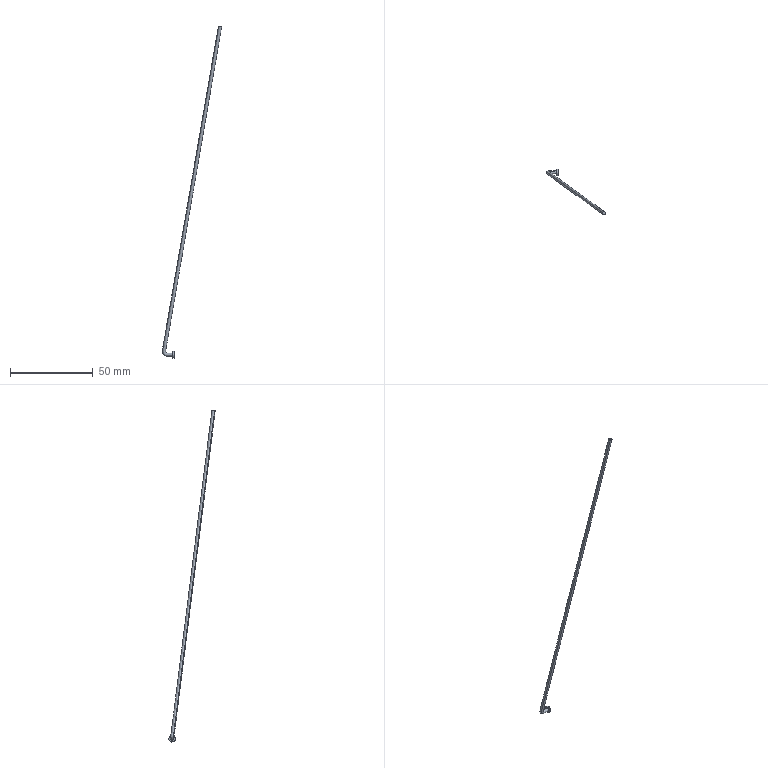Part | STEP file | BREP_61 | 1 solid | 7 faces | box 35.925 x 28.108 x 200.702 mm | volume 653.861 mm3 | plane 3 | spline 2 | cylinder 2 | commonest cylinder face diameters 4 x2
STEP:
#1=CARTESIAN_POINT('',(0.,0.,0.));
#2=DIRECTION('',(0.,0.,1.));
#3=DIRECTION('',(1.,0.,0.));
#4=AXIS2_PLACEMENT_3D('',#1,#2,#3);
#5=CARTESIAN_POINT('',(-13.811,0.6169,212.934));
#6=VERTEX_POINT('',#5);
#7=CARTESIAN_POINT('',(-43.38,25.615,15.366));
#8=VERTEX_POINT('',#7);
#9=CARTESIAN_POINT('',(-13.811,0.6169,212.934));
#10=CARTESIAN_POINT('',(-14.915,1.425,206.549));
#11=CARTESIAN_POINT('',(-17.123,3.041,193.777));
#12=CARTESIAN_POINT('',(-20.435,5.465,174.62));
#13=CARTESIAN_POINT('',(-23.747,7.889,155.462));
#14=CARTESIAN_POINT('',(-27.059,10.313,136.305));
#15=CARTESIAN_POINT('',(-30.371,12.737,117.147));
#16=CARTESIAN_POINT('',(-34.787,15.969,91.603));
#17=CARTESIAN_POINT('',(-38.375,18.594,70.85));
#18=CARTESIAN_POINT('',(-41.135,20.614,54.885));
#19=CARTESIAN_POINT('',(-41.963,21.22,50.096));
#20=CARTESIAN_POINT('',(-42.791,21.826,45.306));
#21=CARTESIAN_POINT('',(-43.619,22.432,40.517));
#22=CARTESIAN_POINT('',(-44.447,23.038,35.728));
#23=CARTESIAN_POINT('',(-45.275,23.644,30.939));
#24=CARTESIAN_POINT('',(-46.104,24.25,26.149));
#25=CARTESIAN_POINT('',(-46.789,24.752,22.184));
#26=CARTESIAN_POINT('',(-47.266,25.101,19.426));
#27=CARTESIAN_POINT('',(-47.531,25.296,17.889));
#28=CARTESIAN_POINT('',(-47.672,25.398,17.08));
#29=CARTESIAN_POINT('',(-47.734,25.445,16.711));
#30=CARTESIAN_POINT('',(-47.738,25.448,16.68));
#31=CARTESIAN_POINT('',(-47.742,25.454,16.637));
#32=CARTESIAN_POINT('',(-47.746,25.467,16.536));
#33=CARTESIAN_POINT('',(-47.736,25.486,16.382));
#34=CARTESIAN_POINT('',(-47.672,25.52,16.116));
#35=CARTESIAN_POINT('',(-47.542,25.55,15.874));
#36=CARTESIAN_POINT('',(-47.357,25.576,15.675));
#37=CARTESIAN_POINT('',(-47.222,25.589,15.572));
#38=CARTESIAN_POINT('',(-47.104,25.597,15.504));
#39=CARTESIAN_POINT('',(-47.01,25.603,15.459));
#40=CARTESIAN_POINT('',(-46.913,25.607,15.423));
#41=CARTESIAN_POINT('',(-46.83,25.61,15.4));
#42=CARTESIAN_POINT('',(-46.764,25.612,15.386));
#43=CARTESIAN_POINT('',(-46.695,25.614,15.375));
#44=CARTESIAN_POINT('',(-46.612,25.615,15.366));
#45=CARTESIAN_POINT('',(-46.467,25.615,15.366));
#46=CARTESIAN_POINT('',(-46.184,25.615,15.366));
#47=CARTESIAN_POINT('',(-45.574,25.615,15.366));
#48=CARTESIAN_POINT('',(-44.614,25.615,15.366));
#49=CARTESIAN_POINT('',(-43.792,25.615,15.366));
#50=CARTESIAN_POINT('',(-43.38,25.615,15.366));
#51=B_SPLINE_CURVE_WITH_KNOTS('',3,(#9,#10,#11,#12,#13,#14,#15,#16,#17,#18,#19,#20,#21,#22,#23,#24,#25,#26,#27,#28,#29,#30,#31,#32,#33,#34,#35,#36,#37,#38,#39,#40,#41,#42,#43,#44,#45,#46,#47,#48,#49,#50),.UNSPECIFIED.,.F.,.F.,(4,1,1,1,1,1,1,1,1,1,1,1,1,1,1,1,1,1,1,1,1,1,1,1,1,1,1,1,1,1,1,1,1,1,1,1,1,1,1,4),(0.,0.09453,0.1891,0.2836,0.3781,0.4726,0.5672,0.7562,0.7798,0.8035,0.8271,0.8507,0.8744,0.898,0.9216,0.9453,0.9567,0.9624,0.9681,0.9684,0.9686,0.969,0.9694,0.971,0.9727,0.976,0.9776,0.9792,0.9801,0.9809,0.9817,0.9825,0.983,0.9834,0.9842,0.9852,0.9861,0.9881,0.994,1.),.UNSPECIFIED.);
#52=CARTESIAN_POINT('',(-41.32,24.739,13.577));
#53=CARTESIAN_POINT('',(-42.412,24.739,13.578));
#54=CARTESIAN_POINT('',(-43.927,24.739,13.578));
#55=CARTESIAN_POINT('',(-45.571,24.739,13.578));
#56=CARTESIAN_POINT('',(-46.19,24.739,13.578));
#57=CARTESIAN_POINT('',(-46.446,24.739,13.578));
#58=CARTESIAN_POINT('',(-46.689,24.739,13.577));
#59=CARTESIAN_POINT('',(-46.913,24.737,13.6));
#60=CARTESIAN_POINT('',(-47.072,24.733,13.626));
#61=CARTESIAN_POINT('',(-47.231,24.729,13.659));
#62=CARTESIAN_POINT('',(-47.429,24.722,13.714));
#63=CARTESIAN_POINT('',(-47.66,24.711,13.8));
#64=CARTESIAN_POINT('',(-47.884,24.698,13.905));
#65=CARTESIAN_POINT('',(-48.165,24.677,14.069));
#66=CARTESIAN_POINT('',(-48.486,24.646,14.315));
#67=CARTESIAN_POINT('',(-48.927,24.586,14.789));
#68=CARTESIAN_POINT('',(-49.238,24.513,15.366));
#69=CARTESIAN_POINT('',(-49.39,24.433,15.998));
#70=CARTESIAN_POINT('',(-49.414,24.387,16.365));
#71=CARTESIAN_POINT('',(-49.403,24.356,16.607));
#72=CARTESIAN_POINT('',(-49.394,24.343,16.706));
#73=CARTESIAN_POINT('',(-49.385,24.333,16.79));
#74=CARTESIAN_POINT('',(-49.307,24.274,17.256));
#75=CARTESIAN_POINT('',(-49.174,24.178,18.017));
#76=CARTESIAN_POINT('',(-48.906,23.981,19.572));
#77=CARTESIAN_POINT('',(-48.43,23.633,22.325));
#78=CARTESIAN_POINT('',(-47.744,23.131,26.291));
#79=CARTESIAN_POINT('',(-46.916,22.525,31.08));
#80=CARTESIAN_POINT('',(-46.088,21.919,35.87));
#81=CARTESIAN_POINT('',(-45.26,21.313,40.659));
#82=CARTESIAN_POINT('',(-44.432,20.707,45.448));
#83=CARTESIAN_POINT('',(-43.604,20.101,50.238));
#84=CARTESIAN_POINT('',(-42.776,19.495,55.027));
#85=CARTESIAN_POINT('',(-40.016,17.475,70.992));
#86=CARTESIAN_POINT('',(-36.428,14.849,91.745));
#87=CARTESIAN_POINT('',(-32.012,11.617,117.289));
#88=CARTESIAN_POINT('',(-28.7,9.193,136.447));
#89=CARTESIAN_POINT('',(-25.388,6.769,155.604));
#90=CARTESIAN_POINT('',(-22.075,4.345,174.762));
#91=CARTESIAN_POINT('',(-18.647,1.836,194.594));
#92=CARTESIAN_POINT('',(-16.322,0.1343,208.042));
#93=CARTESIAN_POINT('',(-15.101,-0.7592,215.103));
#94=CARTESIAN_POINT('',(-41.319,24.491,13.658));
#95=CARTESIAN_POINT('',(-42.413,24.491,13.658));
#96=CARTESIAN_POINT('',(-43.927,24.491,13.658));
#97=CARTESIAN_POINT('',(-45.571,24.491,13.658));
#98=CARTESIAN_POINT('',(-46.189,24.491,13.658));
#99=CARTESIAN_POINT('',(-46.447,24.491,13.658));
#100=CARTESIAN_POINT('',(-46.684,24.492,13.658));
#101=CARTESIAN_POINT('',(-46.899,24.489,13.68));
#102=CARTESIAN_POINT('',(-47.051,24.486,13.705));
#103=CARTESIAN_POINT('',(-47.204,24.482,13.737));
#104=CARTESIAN_POINT('',(-47.395,24.475,13.79));
#105=CARTESIAN_POINT('',(-47.617,24.464,13.872));
#106=CARTESIAN_POINT('',(-47.832,24.452,13.973));
#107=CARTESIAN_POINT('',(-48.102,24.432,14.131));
#108=CARTESIAN_POINT('',(-48.411,24.402,14.367));
#109=CARTESIAN_POINT('',(-48.835,24.344,14.823));
#110=CARTESIAN_POINT('',(-49.133,24.274,15.377));
#111=CARTESIAN_POINT('',(-49.28,24.197,15.985));
#112=CARTESIAN_POINT('',(-49.302,24.152,16.338));
#113=CARTESIAN_POINT('',(-49.292,24.123,16.571));
#114=CARTESIAN_POINT('',(-49.284,24.111,16.666));
#115=CARTESIAN_POINT('',(-49.274,24.101,16.746));
#116=CARTESIAN_POINT('',(-49.198,24.043,17.205));
#117=CARTESIAN_POINT('',(-49.064,23.946,17.969));
#118=CARTESIAN_POINT('',(-48.796,23.749,19.523));
#119=CARTESIAN_POINT('',(-48.32,23.401,22.277));
#120=CARTESIAN_POINT('',(-47.634,22.899,26.243));
#121=CARTESIAN_POINT('',(-46.806,22.293,31.032));
#122=CARTESIAN_POINT('',(-45.978,21.687,35.822));
#123=CARTESIAN_POINT('',(-45.15,21.081,40.611));
#124=CARTESIAN_POINT('',(-44.322,20.475,45.4));
#125=CARTESIAN_POINT('',(-43.494,19.869,50.19));
#126=CARTESIAN_POINT('',(-42.666,19.263,54.979));
#127=CARTESIAN_POINT('',(-39.906,17.243,70.944));
#128=CARTESIAN_POINT('',(-36.318,14.617,91.697));
#129=CARTESIAN_POINT('',(-31.902,11.385,117.241));
#130=CARTESIAN_POINT('',(-28.59,8.961,136.399));
#131=CARTESIAN_POINT('',(-25.278,6.538,155.555));
#132=CARTESIAN_POINT('',(-21.966,4.114,174.713));
#133=CARTESIAN_POINT('',(-18.537,1.604,194.546));
#134=CARTESIAN_POINT('',(-16.212,-0.09729,207.993));
#135=CARTESIAN_POINT('',(-14.991,-0.9907,215.055));
#136=CARTESIAN_POINT('',(-41.313,24.025,14.164));
#137=CARTESIAN_POINT('',(-42.414,24.025,14.164));
#138=CARTESIAN_POINT('',(-43.926,24.025,14.164));
#139=CARTESIAN_POINT('',(-45.572,24.025,14.164));
#140=CARTESIAN_POINT('',(-46.187,24.025,14.164));
#141=CARTESIAN_POINT('',(-46.454,24.025,14.164));
#142=CARTESIAN_POINT('',(-46.658,24.025,14.163));
#143=CARTESIAN_POINT('',(-46.825,24.023,14.181));
#144=CARTESIAN_POINT('',(-46.948,24.02,14.201));
#145=CARTESIAN_POINT('',(-47.069,24.017,14.226));
#146=CARTESIAN_POINT('',(-47.221,24.011,14.268));
#147=CARTESIAN_POINT('',(-47.398,24.003,14.334));
#148=CARTESIAN_POINT('',(-47.569,23.993,14.415));
#149=CARTESIAN_POINT('',(-47.785,23.977,14.54));
#150=CARTESIAN_POINT('',(-48.031,23.953,14.728));
#151=CARTESIAN_POINT('',(-48.369,23.907,15.091));
#152=CARTESIAN_POINT('',(-48.607,23.851,15.533));
#153=CARTESIAN_POINT('',(-48.723,23.79,16.018));
#154=CARTESIAN_POINT('',(-48.741,23.755,16.299));
#155=CARTESIAN_POINT('',(-48.733,23.731,16.484));
#156=CARTESIAN_POINT('',(-48.726,23.721,16.561));
#157=CARTESIAN_POINT('',(-48.719,23.714,16.623));
#158=CARTESIAN_POINT('',(-48.648,23.66,17.05));
#159=CARTESIAN_POINT('',(-48.512,23.561,17.83));
#160=CARTESIAN_POINT('',(-48.244,23.365,19.378));
#161=CARTESIAN_POINT('',(-47.768,23.016,22.133));
#162=CARTESIAN_POINT('',(-47.082,22.515,26.099));
#163=CARTESIAN_POINT('',(-46.254,21.909,30.888));
#164=CARTESIAN_POINT('',(-45.426,21.303,35.677));
#165=CARTESIAN_POINT('',(-44.598,20.697,40.467));
#166=CARTESIAN_POINT('',(-43.77,20.091,45.256));
#167=CARTESIAN_POINT('',(-42.942,19.485,50.046));
#168=CARTESIAN_POINT('',(-42.114,18.879,54.835));
#169=CARTESIAN_POINT('',(-39.354,16.859,70.8));
#170=CARTESIAN_POINT('',(-35.766,14.233,91.553));
#171=CARTESIAN_POINT('',(-31.35,11.001,117.097));
#172=CARTESIAN_POINT('',(-28.038,8.577,136.255));
#173=CARTESIAN_POINT('',(-24.726,6.153,155.411));
#174=CARTESIAN_POINT('',(-21.414,3.729,174.569));
#175=CARTESIAN_POINT('',(-17.985,1.22,194.402));
#176=CARTESIAN_POINT('',(-15.66,-0.4819,207.849));
#177=CARTESIAN_POINT('',(-14.44,-1.375,214.911));
#178=CARTESIAN_POINT('',(-41.304,24.161,15.051));
#179=CARTESIAN_POINT('',(-42.417,24.161,15.051));
#180=CARTESIAN_POINT('',(-43.924,24.161,15.051));
#181=CARTESIAN_POINT('',(-45.573,24.161,15.051));
#182=CARTESIAN_POINT('',(-46.184,24.161,15.051));
#183=CARTESIAN_POINT('',(-46.465,24.161,15.051));
#184=CARTESIAN_POINT('',(-46.618,24.161,15.051));
#185=CARTESIAN_POINT('',(-46.712,24.159,15.061));
#186=CARTESIAN_POINT('',(-46.788,24.158,15.073));
#187=CARTESIAN_POINT('',(-46.861,24.156,15.089));
#188=CARTESIAN_POINT('',(-46.954,24.153,15.114));
#189=CARTESIAN_POINT('',(-47.061,24.147,15.154));
#190=CARTESIAN_POINT('',(-47.165,24.141,15.203));
#191=CARTESIAN_POINT('',(-47.296,24.132,15.279));
#192=CARTESIAN_POINT('',(-47.445,24.117,15.394));
#193=CARTESIAN_POINT('',(-47.65,24.089,15.614));
#194=CARTESIAN_POINT('',(-47.795,24.055,15.882));
#195=CARTESIAN_POINT('',(-47.866,24.018,16.177));
#196=CARTESIAN_POINT('',(-47.876,23.997,16.347));
#197=CARTESIAN_POINT('',(-47.871,23.982,16.46));
#198=CARTESIAN_POINT('',(-47.867,23.976,16.507));
#199=CARTESIAN_POINT('',(-47.863,23.972,16.541));
#200=CARTESIAN_POINT('',(-47.8,23.924,16.918));
#201=CARTESIAN_POINT('',(-47.66,23.822,17.723));
#202=CARTESIAN_POINT('',(-47.394,23.628,19.262));
#203=CARTESIAN_POINT('',(-46.917,23.279,22.02));
#204=CARTESIAN_POINT('',(-46.232,22.777,25.985));
#205=CARTESIAN_POINT('',(-45.404,22.171,30.774));
#206=CARTESIAN_POINT('',(-44.576,21.565,35.564));
#207=CARTESIAN_POINT('',(-43.748,20.959,40.353));
#208=CARTESIAN_POINT('',(-42.92,20.353,45.142));
#209=CARTESIAN_POINT('',(-42.092,19.747,49.932));
#210=CARTESIAN_POINT('',(-41.264,19.141,54.721));
#211=CARTESIAN_POINT('',(-38.503,17.121,70.686));
#212=CARTESIAN_POINT('',(-34.916,14.495,91.439));
#213=CARTESIAN_POINT('',(-30.499,11.263,116.983));
#214=CARTESIAN_POINT('',(-27.187,8.839,136.141));
#215=CARTESIAN_POINT('',(-23.875,6.415,155.297));
#216=CARTESIAN_POINT('',(-20.563,3.991,174.456));
#217=CARTESIAN_POINT('',(-17.134,1.482,194.288));
#218=CARTESIAN_POINT('',(-14.81,-0.2194,207.735));
#219=CARTESIAN_POINT('',(-13.589,-1.113,214.797));
#220=CARTESIAN_POINT('',(-41.299,24.858,15.61));
#221=CARTESIAN_POINT('',(-42.419,24.858,15.61));
#222=CARTESIAN_POINT('',(-43.923,24.858,15.61));
#223=CARTESIAN_POINT('',(-45.574,24.858,15.61));
#224=CARTESIAN_POINT('',(-46.183,24.858,15.61));
#225=CARTESIAN_POINT('',(-46.471,24.858,15.61));
#226=CARTESIAN_POINT('',(-46.596,24.858,15.609));
#227=CARTESIAN_POINT('',(-46.65,24.857,15.616));
#228=CARTESIAN_POINT('',(-46.701,24.856,15.624));
#229=CARTESIAN_POINT('',(-46.749,24.855,15.634));
#230=CARTESIAN_POINT('',(-46.809,24.853,15.651));
#231=CARTESIAN_POINT('',(-46.879,24.849,15.677));
#232=CARTESIAN_POINT('',(-46.946,24.845,15.709));
#233=CARTESIAN_POINT('',(-47.031,24.839,15.758));
#234=CARTESIAN_POINT('',(-47.128,24.83,15.832));
#235=CARTESIAN_POINT('',(-47.262,24.812,15.976));
#236=CARTESIAN_POINT('',(-47.356,24.789,16.15));
#237=CARTESIAN_POINT('',(-47.402,24.765,16.341));
#238=CARTESIAN_POINT('',(-47.409,24.751,16.452));
#239=CARTESIAN_POINT('',(-47.405,24.742,16.525));
#240=CARTESIAN_POINT('',(-47.403,24.738,16.557));
#241=CARTESIAN_POINT('',(-47.401,24.736,16.576));
#242=CARTESIAN_POINT('',(-47.341,24.691,16.926));
#243=CARTESIAN_POINT('',(-47.199,24.588,17.745));
#244=CARTESIAN_POINT('',(-46.934,24.394,19.278));
#245=CARTESIAN_POINT('',(-46.457,24.045,22.038));
#246=CARTESIAN_POINT('',(-45.772,23.543,26.002));
#247=CARTESIAN_POINT('',(-44.944,22.937,30.792));
#248=CARTESIAN_POINT('',(-44.116,22.331,35.581));
#249=CARTESIAN_POINT('',(-43.288,21.725,40.37));
#250=CARTESIAN_POINT('',(-42.46,21.119,45.159));
#251=CARTESIAN_POINT('',(-41.631,20.513,49.949));
#252=CARTESIAN_POINT('',(-40.804,19.907,54.738));
#253=CARTESIAN_POINT('',(-38.043,17.887,70.703));
#254=CARTESIAN_POINT('',(-34.455,15.261,91.456));
#255=CARTESIAN_POINT('',(-30.039,12.029,117.));
#256=CARTESIAN_POINT('',(-26.727,9.605,136.158));
#257=CARTESIAN_POINT('',(-23.415,7.181,155.315));
#258=CARTESIAN_POINT('',(-20.103,4.757,174.473));
#259=CARTESIAN_POINT('',(-16.674,2.248,194.305));
#260=CARTESIAN_POINT('',(-14.349,0.5465,207.753));
#261=CARTESIAN_POINT('',(-13.129,-0.347,214.814));
#262=CARTESIAN_POINT('',(-41.301,25.523,15.463));
#263=CARTESIAN_POINT('',(-42.418,25.523,15.463));
#264=CARTESIAN_POINT('',(-43.923,25.523,15.463));
#265=CARTESIAN_POINT('',(-45.574,25.523,15.463));
#266=CARTESIAN_POINT('',(-46.183,25.523,15.463));
#267=CARTESIAN_POINT('',(-46.468,25.523,15.463));
#268=CARTESIAN_POINT('',(-46.607,25.523,15.462));
#269=CARTESIAN_POINT('',(-46.681,25.522,15.471));
#270=CARTESIAN_POINT('',(-46.744,25.521,15.481));
#271=CARTESIAN_POINT('',(-46.804,25.519,15.494));
#272=CARTESIAN_POINT('',(-46.88,25.517,15.515));
#273=CARTESIAN_POINT('',(-46.968,25.513,15.547));
#274=CARTESIAN_POINT('',(-47.054,25.507,15.588));
#275=CARTESIAN_POINT('',(-47.161,25.5,15.65));
#276=CARTESIAN_POINT('',(-47.284,25.488,15.744));
#277=CARTESIAN_POINT('',(-47.453,25.465,15.926));
#278=CARTESIAN_POINT('',(-47.571,25.437,16.146));
#279=CARTESIAN_POINT('',(-47.63,25.406,16.388));
#280=CARTESIAN_POINT('',(-47.639,25.388,16.528));
#281=CARTESIAN_POINT('',(-47.635,25.377,16.62));
#282=CARTESIAN_POINT('',(-47.631,25.372,16.66));
#283=CARTESIAN_POINT('',(-47.628,25.368,16.687));
#284=CARTESIAN_POINT('',(-47.566,25.322,17.05));
#285=CARTESIAN_POINT('',(-47.426,25.22,17.862));
#286=CARTESIAN_POINT('',(-47.16,25.025,19.398));
#287=CARTESIAN_POINT('',(-46.683,24.676,22.157));
#288=CARTESIAN_POINT('',(-45.998,24.175,26.121));
#289=CARTESIAN_POINT('',(-45.17,23.569,30.911));
#290=CARTESIAN_POINT('',(-44.342,22.963,35.7));
#291=CARTESIAN_POINT('',(-43.514,22.357,40.489));
#292=CARTESIAN_POINT('',(-42.686,21.751,45.278));
#293=CARTESIAN_POINT('',(-41.858,21.145,50.068));
#294=CARTESIAN_POINT('',(-41.03,20.539,54.857));
#295=CARTESIAN_POINT('',(-38.27,18.519,70.822));
#296=CARTESIAN_POINT('',(-34.682,15.893,91.576));
#297=CARTESIAN_POINT('',(-30.266,12.661,117.119));
#298=CARTESIAN_POINT('',(-26.953,10.237,136.277));
#299=CARTESIAN_POINT('',(-23.641,7.813,155.434));
#300=CARTESIAN_POINT('',(-20.329,5.389,174.592));
#301=CARTESIAN_POINT('',(-16.901,2.88,194.424));
#302=CARTESIAN_POINT('',(-14.576,1.178,207.872));
#303=CARTESIAN_POINT('',(-13.355,0.2847,214.933));
#304=CARTESIAN_POINT('',(-41.303,25.719,15.292));
#305=CARTESIAN_POINT('',(-42.417,25.719,15.293));
#306=CARTESIAN_POINT('',(-43.924,25.719,15.292));
#307=CARTESIAN_POINT('',(-45.574,25.719,15.293));
#308=CARTESIAN_POINT('',(-46.184,25.719,15.292));
#309=CARTESIAN_POINT('',(-46.465,25.719,15.293));
#310=CARTESIAN_POINT('',(-46.616,25.719,15.292));
#311=CARTESIAN_POINT('',(-46.706,25.718,15.302));
#312=CARTESIAN_POINT('',(-46.78,25.716,15.314));
#313=CARTESIAN_POINT('',(-46.851,25.714,15.329));
#314=CARTESIAN_POINT('',(-46.94,25.711,15.354));
#315=CARTESIAN_POINT('',(-47.044,25.706,15.392));
#316=CARTESIAN_POINT('',(-47.144,25.7,15.44));
#317=CARTESIAN_POINT('',(-47.271,25.691,15.513));
#318=CARTESIAN_POINT('',(-47.415,25.677,15.624));
#319=CARTESIAN_POINT('',(-47.614,25.65,15.837));
#320=CARTESIAN_POINT('',(-47.753,25.617,16.096));
#321=CARTESIAN_POINT('',(-47.822,25.581,16.381));
#322=CARTESIAN_POINT('',(-47.832,25.56,16.546));
#323=CARTESIAN_POINT('',(-47.827,25.547,16.655));
#324=CARTESIAN_POINT('',(-47.823,25.541,16.7));
#325=CARTESIAN_POINT('',(-47.82,25.537,16.734));
#326=CARTESIAN_POINT('',(-47.756,25.489,17.108));
#327=CARTESIAN_POINT('',(-47.616,25.387,17.914));
#328=CARTESIAN_POINT('',(-47.351,25.193,19.452));
#329=CARTESIAN_POINT('',(-46.874,24.844,22.211));
#330=CARTESIAN_POINT('',(-46.188,24.342,26.175));
#331=CARTESIAN_POINT('',(-45.36,23.736,30.965));
#332=CARTESIAN_POINT('',(-44.532,23.13,35.754));
#333=CARTESIAN_POINT('',(-43.704,22.524,40.543));
#334=CARTESIAN_POINT('',(-42.876,21.918,45.332));
#335=CARTESIAN_POINT('',(-42.048,21.312,50.122));
#336=CARTESIAN_POINT('',(-41.22,20.706,54.911));
#337=CARTESIAN_POINT('',(-38.46,18.686,70.876));
#338=CARTESIAN_POINT('',(-34.872,16.06,91.63));
#339=CARTESIAN_POINT('',(-30.456,12.828,117.173));
#340=CARTESIAN_POINT('',(-27.144,10.404,136.331));
#341=CARTESIAN_POINT('',(-23.832,7.98,155.488));
#342=CARTESIAN_POINT('',(-20.52,5.556,174.646));
#343=CARTESIAN_POINT('',(-17.091,3.047,194.478));
#344=CARTESIAN_POINT('',(-14.766,1.345,207.926));
#345=CARTESIAN_POINT('',(-13.545,0.452,214.987));
#346=B_SPLINE_SURFACE_WITH_KNOTS('',3,3,((#52,#53,#54,#55,#56,#57,#58,#59,#60,#61,#62,#63,#64,#65,#66,#67,#68,#69,#70,#71,#72,#73,#74,#75,#76,#77,#78,#79,#80,#81,#82,#83,#84,#85,#86,#87,#88,#89,#90,#91,#92,#93),(#94,#95,#96,#97,#98,#99,#100,#101,#102,#103,#104,#105,#106,#107,#108,#109,#110,#111,#112,#113,#114,#115,#116,#117,#118,#119,#120,#121,#122,#123,#124,#125,#126,#127,#128,#129,#130,#131,#132,#133,#134,#135),(#136,#137,#138,#139,#140,#141,#142,#143,#144,#145,#146,#147,#148,#149,#150,#151,#152,#153,#154,#155,#156,#157,#158,#159,#160,#161,#162,#163,#164,#165,#166,#167,#168,#169,#170,#171,#172,#173,#174,#175,#176,#177),(#178,#179,#180,#181,#182,#183,#184,#185,#186,#187,#188,#189,#190,#191,#192,#193,#194,#195,#196,#197,#198,#199,#200,#201,#202,#203,#204,#205,#206,#207,#208,#209,#210,#211,#212,#213,#214,#215,#216,#217,#218,#219),(#220,#221,#222,#223,#224,#225,#226,#227,#228,#229,#230,#231,#232,#233,#234,#235,#236,#237,#238,#239,#240,#241,#242,#243,#244,#245,#246,#247,#248,#249,#250,#251,#252,#253,#254,#255,#256,#257,#258,#259,#260,#261),(#262,#263,#264,#265,#266,#267,#268,#269,#270,#271,#272,#273,#274,#275,#276,#277,#278,#279,#280,#281,#282,#283,#284,#285,#286,#287,#288,#289,#290,#291,#292,#293,#294,#295,#296,#297,#298,#299,#300,#301,#302,#303),(#304,#305,#306,#307,#308,#309,#310,#311,#312,#313,#314,#315,#316,#317,#318,#319,#320,#321,#322,#323,#324,#325,#326,#327,#328,#329,#330,#331,#332,#333,#334,#335,#336,#337,#338,#339,#340,#341,#342,#343,#344,#345)),.UNSPECIFIED.,.F.,.F.,.F.,(4,1,1,1,4),(4,1,1,1,1,1,1,1,1,1,1,1,1,1,1,1,1,1,1,1,1,1,1,1,1,1,1,1,1,1,1,1,1,1,1,1,1,1,1,4),(-3.3,-2.356,-1.571,-0.7854,0.1472),(-2.066,1.234,2.469,2.874,3.077,3.279,3.448,3.533,3.617,3.79,3.962,4.134,4.306,4.643,4.98,5.661,6.004,6.347,6.431,6.515,6.559,6.602,7.787,8.973,11.344,16.242,21.14,26.038,30.936,35.834,40.732,45.63,50.528,89.712,109.305,128.897,148.489,168.081,187.673,209.338),.UNSPECIFIED.);
#347=CARTESIAN_POINT('',(0.,207.265));
#348=CARTESIAN_POINT('',(0.,0.));
#349=B_SPLINE_CURVE_WITH_KNOTS('',1,(#347,#348),.UNSPECIFIED.,.F.,.F.,(2,2),(0.,1.),.PIECEWISE_BEZIER_KNOTS.);
#350=(GEOMETRIC_REPRESENTATION_CONTEXT(2)PARAMETRIC_REPRESENTATION_CONTEXT()REPRESENTATION_CONTEXT('',''));
#351=DEFINITIONAL_REPRESENTATION('',(#349),#350);
#352=PCURVE('',#346,#351);
#353=CARTESIAN_POINT('',(-41.301,25.49,15.422));
#354=CARTESIAN_POINT('',(-42.417,25.49,15.422));
#355=CARTESIAN_POINT('',(-43.923,25.49,15.422));
#356=CARTESIAN_POINT('',(-45.574,25.49,15.422));
#357=CARTESIAN_POINT('',(-46.184,25.49,15.422));
#358=CARTESIAN_POINT('',(-46.467,25.49,15.422));
#359=CARTESIAN_POINT('',(-46.609,25.49,15.422));
#360=CARTESIAN_POINT('',(-46.685,25.489,15.431));
#361=CARTESIAN_POINT('',(-46.75,25.488,15.442));
#362=CARTESIAN_POINT('',(-46.813,25.486,15.455));
#363=CARTESIAN_POINT('',(-46.891,25.483,15.476));
#364=CARTESIAN_POINT('',(-46.982,25.479,15.51));
#365=CARTESIAN_POINT('',(-47.071,25.474,15.552));
#366=CARTESIAN_POINT('',(-47.182,25.466,15.616));
#367=CARTESIAN_POINT('',(-47.308,25.453,15.713));
#368=CARTESIAN_POINT('',(-47.482,25.43,15.9));
#369=CARTESIAN_POINT('',(-47.605,25.401,16.128));
#370=CARTESIAN_POINT('',(-47.665,25.369,16.378));
#371=CARTESIAN_POINT('',(-47.674,25.351,16.523));
#372=CARTESIAN_POINT('',(-47.67,25.339,16.618));
#373=CARTESIAN_POINT('',(-47.666,25.334,16.659));
#374=CARTESIAN_POINT('',(-47.663,25.33,16.687));
#375=CARTESIAN_POINT('',(-47.601,25.284,17.052));
#376=CARTESIAN_POINT('',(-47.461,25.181,17.863));
#377=CARTESIAN_POINT('',(-47.195,24.987,19.399));
#378=CARTESIAN_POINT('',(-46.718,24.638,22.158));
#379=CARTESIAN_POINT('',(-46.033,24.136,26.122));
#380=CARTESIAN_POINT('',(-45.205,23.53,30.912));
#381=CARTESIAN_POINT('',(-44.377,22.924,35.701));
#382=CARTESIAN_POINT('',(-43.549,22.318,40.491));
#383=CARTESIAN_POINT('',(-42.721,21.712,45.28));
#384=CARTESIAN_POINT('',(-41.893,21.106,50.07));
#385=CARTESIAN_POINT('',(-41.065,20.5,54.859));
#386=CARTESIAN_POINT('',(-38.305,18.48,70.824));
#387=CARTESIAN_POINT('',(-34.717,15.854,91.577));
#388=CARTESIAN_POINT('',(-30.301,12.623,117.12));
#389=CARTESIAN_POINT('',(-26.989,10.198,136.278));
#390=CARTESIAN_POINT('',(-23.677,7.775,155.435));
#391=CARTESIAN_POINT('',(-20.364,5.351,174.593));
#392=CARTESIAN_POINT('',(-16.936,2.841,194.426));
#393=CARTESIAN_POINT('',(-14.611,1.14,207.873));
#394=CARTESIAN_POINT('',(-13.39,0.2463,214.934));
#395=CARTESIAN_POINT('',(-41.302,25.738,15.342));
#396=CARTESIAN_POINT('',(-42.417,25.738,15.342));
#397=CARTESIAN_POINT('',(-43.923,25.738,15.342));
#398=CARTESIAN_POINT('',(-45.574,25.738,15.342));
#399=CARTESIAN_POINT('',(-46.184,25.738,15.342));
#400=CARTESIAN_POINT('',(-46.466,25.738,15.342));
#401=CARTESIAN_POINT('',(-46.614,25.738,15.341));
#402=CARTESIAN_POINT('',(-46.7,25.737,15.351));
#403=CARTESIAN_POINT('',(-46.771,25.735,15.363));
#404=CARTESIAN_POINT('',(-46.84,25.734,15.377));
#405=CARTESIAN_POINT('',(-46.926,25.731,15.401));
#406=CARTESIAN_POINT('',(-47.026,25.726,15.438));
#407=CARTESIAN_POINT('',(-47.123,25.72,15.484));
#408=CARTESIAN_POINT('',(-47.245,25.711,15.555));
#409=CARTESIAN_POINT('',(-47.384,25.698,15.661));
#410=CARTESIAN_POINT('',(-47.575,25.672,15.867));
#411=CARTESIAN_POINT('',(-47.71,25.64,16.117));
#412=CARTESIAN_POINT('',(-47.776,25.605,16.391));
#413=CARTESIAN_POINT('',(-47.786,25.585,16.55));
#414=CARTESIAN_POINT('',(-47.781,25.572,16.655));
#415=CARTESIAN_POINT('',(-47.777,25.566,16.699));
#416=CARTESIAN_POINT('',(-47.774,25.562,16.731));
#417=CARTESIAN_POINT('',(-47.711,25.515,17.102));
#418=CARTESIAN_POINT('',(-47.571,25.413,17.91));
#419=CARTESIAN_POINT('',(-47.305,25.218,19.448));
#420=CARTESIAN_POINT('',(-46.828,24.869,22.206));
#421=CARTESIAN_POINT('',(-46.143,24.368,26.17));
#422=CARTESIAN_POINT('',(-45.314,23.762,30.96));
#423=CARTESIAN_POINT('',(-44.486,23.156,35.749));
#424=CARTESIAN_POINT('',(-43.658,22.55,40.539));
#425=CARTESIAN_POINT('',(-42.831,21.944,45.328));
#426=CARTESIAN_POINT('',(-42.002,21.338,50.118));
#427=CARTESIAN_POINT('',(-41.174,20.732,54.907));
#428=CARTESIAN_POINT('',(-38.414,18.712,70.872));
#429=CARTESIAN_POINT('',(-34.826,16.086,91.625));
#430=CARTESIAN_POINT('',(-30.41,12.854,117.169));
#431=CARTESIAN_POINT('',(-27.098,10.43,136.327));
#432=CARTESIAN_POINT('',(-23.786,8.006,155.483));
#433=CARTESIAN_POINT('',(-20.474,5.582,174.641));
#434=CARTESIAN_POINT('',(-17.045,3.073,194.474));
#435=CARTESIAN_POINT('',(-14.72,1.371,207.921));
#436=CARTESIAN_POINT('',(-13.5,0.4779,214.983));
#437=CARTESIAN_POINT('',(-41.308,26.205,14.836));
#438=CARTESIAN_POINT('',(-42.415,26.205,14.836));
#439=CARTESIAN_POINT('',(-43.924,26.205,14.836));
#440=CARTESIAN_POINT('',(-45.573,26.205,14.836));
#441=CARTESIAN_POINT('',(-46.186,26.205,14.836));
#442=CARTESIAN_POINT('',(-46.459,26.205,14.836));
#443=CARTESIAN_POINT('',(-46.64,26.205,14.836));
#444=CARTESIAN_POINT('',(-46.773,26.203,14.85));
#445=CARTESIAN_POINT('',(-46.875,26.201,14.867));
#446=CARTESIAN_POINT('',(-46.975,26.198,14.888));
#447=CARTESIAN_POINT('',(-47.099,26.194,14.922));
#448=CARTESIAN_POINT('',(-47.244,26.187,14.976));
#449=CARTESIAN_POINT('',(-47.385,26.179,15.042));
#450=CARTESIAN_POINT('',(-47.562,26.166,15.145));
#451=CARTESIAN_POINT('',(-47.764,26.146,15.3));
#452=CARTESIAN_POINT('',(-48.041,26.108,15.598));
#453=CARTESIAN_POINT('',(-48.236,26.063,15.961));
#454=CARTESIAN_POINT('',(-48.332,26.012,16.358));
#455=CARTESIAN_POINT('',(-48.347,25.983,16.589));
#456=CARTESIAN_POINT('',(-48.34,25.964,16.741));
#457=CARTESIAN_POINT('',(-48.334,25.956,16.804));
#458=CARTESIAN_POINT('',(-48.329,25.95,16.854));
#459=CARTESIAN_POINT('',(-48.261,25.898,17.258));
#460=CARTESIAN_POINT('',(-48.123,25.798,18.049));
#461=CARTESIAN_POINT('',(-47.857,25.603,19.593));
#462=CARTESIAN_POINT('',(-47.38,25.254,22.349));
#463=CARTESIAN_POINT('',(-46.694,24.752,26.315));
#464=CARTESIAN_POINT('',(-45.866,24.146,31.104));
#465=CARTESIAN_POINT('',(-45.038,23.54,35.894));
#466=CARTESIAN_POINT('',(-44.21,22.934,40.683));
#467=CARTESIAN_POINT('',(-43.382,22.329,45.472));
#468=CARTESIAN_POINT('',(-42.554,21.722,50.262));
#469=CARTESIAN_POINT('',(-41.726,21.117,55.051));
#470=CARTESIAN_POINT('',(-38.966,19.097,71.016));
#471=CARTESIAN_POINT('',(-35.378,16.471,91.769));
#472=CARTESIAN_POINT('',(-30.962,13.239,117.313));
#473=CARTESIAN_POINT('',(-27.65,10.815,136.471));
#474=CARTESIAN_POINT('',(-24.338,8.391,155.627));
#475=CARTESIAN_POINT('',(-21.026,5.967,174.785));
#476=CARTESIAN_POINT('',(-17.597,3.457,194.618));
#477=CARTESIAN_POINT('',(-15.272,1.756,208.065));
#478=CARTESIAN_POINT('',(-14.051,0.8625,215.127));
#479=CARTESIAN_POINT('',(-41.317,26.069,13.949));
#480=CARTESIAN_POINT('',(-42.412,26.069,13.949));
#481=CARTESIAN_POINT('',(-43.926,26.069,13.949));
#482=CARTESIAN_POINT('',(-45.572,26.069,13.949));
#483=CARTESIAN_POINT('',(-46.189,26.069,13.949));
#484=CARTESIAN_POINT('',(-46.449,26.069,13.949));
#485=CARTESIAN_POINT('',(-46.679,26.069,13.949));
#486=CARTESIAN_POINT('',(-46.887,26.066,13.97));
#487=CARTESIAN_POINT('',(-47.035,26.063,13.994));
#488=CARTESIAN_POINT('',(-47.183,26.059,14.025));
#489=CARTESIAN_POINT('',(-47.367,26.053,14.076));
#490=CARTESIAN_POINT('',(-47.581,26.043,14.156));
#491=CARTESIAN_POINT('',(-47.789,26.03,14.254));
#492=CARTESIAN_POINT('',(-48.051,26.011,14.406));
#493=CARTESIAN_POINT('',(-48.35,25.982,14.634));
#494=CARTESIAN_POINT('',(-48.759,25.926,15.075));
#495=CARTESIAN_POINT('',(-49.048,25.859,15.611));
#496=CARTESIAN_POINT('',(-49.19,25.784,16.2));
#497=CARTESIAN_POINT('',(-49.212,25.741,16.541));
#498=CARTESIAN_POINT('',(-49.202,25.713,16.766));
#499=CARTESIAN_POINT('',(-49.194,25.701,16.858));
#500=CARTESIAN_POINT('',(-49.185,25.691,16.935));
#501=CARTESIAN_POINT('',(-49.109,25.634,17.389));
#502=CARTESIAN_POINT('',(-48.975,25.537,18.156));
#503=CARTESIAN_POINT('',(-48.707,25.34,19.709));
#504=CARTESIAN_POINT('',(-48.231,24.992,22.463));
#505=CARTESIAN_POINT('',(-47.545,24.49,26.429));
#506=CARTESIAN_POINT('',(-46.717,23.884,31.218));
#507=CARTESIAN_POINT('',(-45.889,23.278,36.007));
#508=CARTESIAN_POINT('',(-45.061,22.672,40.797));
#509=CARTESIAN_POINT('',(-44.233,22.066,45.586));
#510=CARTESIAN_POINT('',(-43.405,21.46,50.376));
#511=CARTESIAN_POINT('',(-42.577,20.854,55.165));
#512=CARTESIAN_POINT('',(-39.817,18.834,71.13));
#513=CARTESIAN_POINT('',(-36.229,16.208,91.883));
#514=CARTESIAN_POINT('',(-31.813,12.976,117.426));
#515=CARTESIAN_POINT('',(-28.501,10.552,136.584));
#516=CARTESIAN_POINT('',(-25.189,8.128,155.741));
#517=CARTESIAN_POINT('',(-21.877,5.704,174.899));
#518=CARTESIAN_POINT('',(-18.448,3.195,194.732));
#519=CARTESIAN_POINT('',(-16.123,1.493,208.179));
#520=CARTESIAN_POINT('',(-14.902,0.6,215.241));
#521=CARTESIAN_POINT('',(-41.322,25.372,13.39));
#522=CARTESIAN_POINT('',(-42.411,25.372,13.39));
#523=CARTESIAN_POINT('',(-43.927,25.372,13.39));
#524=CARTESIAN_POINT('',(-45.571,25.372,13.39));
#525=CARTESIAN_POINT('',(-46.19,25.372,13.39));
#526=CARTESIAN_POINT('',(-46.443,25.372,13.391));
#527=CARTESIAN_POINT('',(-46.701,25.372,13.39));
#528=CARTESIAN_POINT('',(-46.948,25.369,13.415));
#529=CARTESIAN_POINT('',(-47.121,25.365,13.443));
#530=CARTESIAN_POINT('',(-47.295,25.36,13.48));
#531=CARTESIAN_POINT('',(-47.511,25.353,13.539));
#532=CARTESIAN_POINT('',(-47.764,25.341,13.633));
#533=CARTESIAN_POINT('',(-48.008,25.326,13.748));
#534=CARTESIAN_POINT('',(-48.316,25.304,13.927));
#535=CARTESIAN_POINT('',(-48.666,25.27,14.196));
#536=CARTESIAN_POINT('',(-49.148,25.204,14.713));
#537=CARTESIAN_POINT('',(-49.487,25.124,15.344));
#538=CARTESIAN_POINT('',(-49.654,25.037,16.035));
#539=CARTESIAN_POINT('',(-49.679,24.986,16.435));
#540=CARTESIAN_POINT('',(-49.668,24.953,16.7));
#541=CARTESIAN_POINT('',(-49.658,24.939,16.808));
#542=CARTESIAN_POINT('',(-49.647,24.927,16.9));
#543=CARTESIAN_POINT('',(-49.568,24.867,17.381));
#544=CARTESIAN_POINT('',(-49.436,24.771,18.135));
#545=CARTESIAN_POINT('',(-49.167,24.574,19.693));
#546=CARTESIAN_POINT('',(-48.691,24.226,22.445));
#547=CARTESIAN_POINT('',(-48.005,23.724,26.412));
#548=CARTESIAN_POINT('',(-47.177,23.118,31.201));
#549=CARTESIAN_POINT('',(-46.349,22.512,35.99));
#550=CARTESIAN_POINT('',(-45.521,21.906,40.779));
#551=CARTESIAN_POINT('',(-44.693,21.3,45.568));
#552=CARTESIAN_POINT('',(-43.865,20.694,50.358));
#553=CARTESIAN_POINT('',(-43.037,20.088,55.147));
#554=CARTESIAN_POINT('',(-40.277,18.068,71.112));
#555=CARTESIAN_POINT('',(-36.689,15.442,91.866));
#556=CARTESIAN_POINT('',(-32.273,12.21,117.409));
#557=CARTESIAN_POINT('',(-28.961,9.786,136.567));
#558=CARTESIAN_POINT('',(-25.649,7.362,155.724));
#559=CARTESIAN_POINT('',(-22.337,4.938,174.882));
#560=CARTESIAN_POINT('',(-18.908,2.429,194.714));
#561=CARTESIAN_POINT('',(-16.583,0.7276,208.162));
#562=CARTESIAN_POINT('',(-15.362,-0.1659,215.223));
#563=CARTESIAN_POINT('',(-41.319,24.706,13.537));
#564=CARTESIAN_POINT('',(-42.411,24.706,13.537));
#565=CARTESIAN_POINT('',(-43.927,24.706,13.537));
#566=CARTESIAN_POINT('',(-45.571,24.706,13.537));
#567=CARTESIAN_POINT('',(-46.19,24.706,13.537));
#568=CARTESIAN_POINT('',(-46.446,24.706,13.538));
#569=CARTESIAN_POINT('',(-46.69,24.706,13.537));
#570=CARTESIAN_POINT('',(-46.918,24.703,13.56));
#571=CARTESIAN_POINT('',(-47.078,24.7,13.587));
#572=CARTESIAN_POINT('',(-47.24,24.696,13.62));
#573=CARTESIAN_POINT('',(-47.44,24.689,13.676));
#574=CARTESIAN_POINT('',(-47.674,24.678,13.762));
#575=CARTESIAN_POINT('',(-47.901,24.664,13.869));
#576=CARTESIAN_POINT('',(-48.186,24.643,14.035));
#577=CARTESIAN_POINT('',(-48.511,24.612,14.284));
#578=CARTESIAN_POINT('',(-48.957,24.551,14.764));
#579=CARTESIAN_POINT('',(-49.271,24.477,15.348));
#580=CARTESIAN_POINT('',(-49.426,24.396,15.988));
#581=CARTESIAN_POINT('',(-49.449,24.349,16.36));
#582=CARTESIAN_POINT('',(-49.439,24.318,16.605));
#583=CARTESIAN_POINT('',(-49.43,24.305,16.705));
#584=CARTESIAN_POINT('',(-49.42,24.295,16.79));
#585=CARTESIAN_POINT('',(-49.342,24.236,17.258));
#586=CARTESIAN_POINT('',(-49.209,24.139,18.018));
#587=CARTESIAN_POINT('',(-48.941,23.943,19.573));
#588=CARTESIAN_POINT('',(-48.465,23.594,22.326));
#589=CARTESIAN_POINT('',(-47.779,23.092,26.292));
#590=CARTESIAN_POINT('',(-46.951,22.486,31.082));
#591=CARTESIAN_POINT('',(-46.123,21.88,35.871));
#592=CARTESIAN_POINT('',(-45.295,21.274,40.66));
#593=CARTESIAN_POINT('',(-44.467,20.668,45.449));
#594=CARTESIAN_POINT('',(-43.639,20.062,50.239));
#595=CARTESIAN_POINT('',(-42.811,19.456,55.028));
#596=CARTESIAN_POINT('',(-40.051,17.436,70.993));
#597=CARTESIAN_POINT('',(-36.463,14.811,91.747));
#598=CARTESIAN_POINT('',(-32.047,11.579,117.29));
#599=CARTESIAN_POINT('',(-28.735,9.155,136.448));
#600=CARTESIAN_POINT('',(-25.423,6.731,155.605));
#601=CARTESIAN_POINT('',(-22.111,4.307,174.763));
#602=CARTESIAN_POINT('',(-18.682,1.797,194.595));
#603=CARTESIAN_POINT('',(-16.357,0.09588,208.043));
#604=CARTESIAN_POINT('',(-15.136,-0.7976,215.104));
#605=CARTESIAN_POINT('',(-41.317,24.511,13.707));
#606=CARTESIAN_POINT('',(-42.412,24.511,13.708));
#607=CARTESIAN_POINT('',(-43.926,24.511,13.707));
#608=CARTESIAN_POINT('',(-45.571,24.511,13.708));
#609=CARTESIAN_POINT('',(-46.189,24.511,13.707));
#610=CARTESIAN_POINT('',(-46.448,24.511,13.708));
#611=CARTESIAN_POINT('',(-46.681,24.511,13.707));
#612=CARTESIAN_POINT('',(-46.893,24.508,13.728));
#613=CARTESIAN_POINT('',(-47.043,24.505,13.753));
#614=CARTESIAN_POINT('',(-47.193,24.501,13.785));
#615=CARTESIAN_POINT('',(-47.38,24.494,13.836));
#616=CARTESIAN_POINT('',(-47.599,24.484,13.917));
#617=CARTESIAN_POINT('',(-47.81,24.471,14.017));
#618=CARTESIAN_POINT('',(-48.076,24.452,14.172));
#619=CARTESIAN_POINT('',(-48.379,24.422,14.404));
#620=CARTESIAN_POINT('',(-48.796,24.366,14.852));
#621=CARTESIAN_POINT('',(-49.09,24.297,15.397));
#622=CARTESIAN_POINT('',(-49.234,24.221,15.995));
#623=CARTESIAN_POINT('',(-49.256,24.177,16.342));
#624=CARTESIAN_POINT('',(-49.246,24.148,16.571));
#625=CARTESIAN_POINT('',(-49.237,24.136,16.665));
#626=CARTESIAN_POINT('',(-49.228,24.127,16.743));
#627=CARTESIAN_POINT('',(-49.152,24.069,17.2));
#628=CARTESIAN_POINT('',(-49.018,23.972,17.965));
#629=CARTESIAN_POINT('',(-48.75,23.775,19.519));
#630=CARTESIAN_POINT('',(-48.274,23.427,22.272));
#631=CARTESIAN_POINT('',(-47.589,22.925,26.238));
#632=CARTESIAN_POINT('',(-46.761,22.319,31.027));
#633=CARTESIAN_POINT('',(-45.933,21.713,35.817));
#634=CARTESIAN_POINT('',(-45.105,21.107,40.606));
#635=CARTESIAN_POINT('',(-44.277,20.501,45.395));
#636=CARTESIAN_POINT('',(-43.448,19.895,50.185));
#637=CARTESIAN_POINT('',(-42.621,19.289,54.974));
#638=CARTESIAN_POINT('',(-39.86,17.269,70.939));
#639=CARTESIAN_POINT('',(-36.272,14.643,91.692));
#640=CARTESIAN_POINT('',(-31.856,11.411,117.236));
#641=CARTESIAN_POINT('',(-28.544,8.987,136.394));
#642=CARTESIAN_POINT('',(-25.232,6.564,155.551));
#643=CARTESIAN_POINT('',(-21.92,4.139,174.709));
#644=CARTESIAN_POINT('',(-18.491,1.63,194.541));
#645=CARTESIAN_POINT('',(-16.166,-0.07136,207.989));
#646=CARTESIAN_POINT('',(-14.946,-0.9648,215.05));
#647=B_SPLINE_SURFACE_WITH_KNOTS('',3,3,((#353,#354,#355,#356,#357,#358,#359,#360,#361,#362,#363,#364,#365,#366,#367,#368,#369,#370,#371,#372,#373,#374,#375,#376,#377,#378,#379,#380,#381,#382,#383,#384,#385,#386,#387,#388,#389,#390,#391,#392,#393,#394),(#395,#396,#397,#398,#399,#400,#401,#402,#403,#404,#405,#406,#407,#408,#409,#410,#411,#412,#413,#414,#415,#416,#417,#418,#419,#420,#421,#422,#423,#424,#425,#426,#427,#428,#429,#430,#431,#432,#433,#434,#435,#436),(#437,#438,#439,#440,#441,#442,#443,#444,#445,#446,#447,#448,#449,#450,#451,#452,#453,#454,#455,#456,#457,#458,#459,#460,#461,#462,#463,#464,#465,#466,#467,#468,#469,#470,#471,#472,#473,#474,#475,#476,#477,#478),(#479,#480,#481,#482,#483,#484,#485,#486,#487,#488,#489,#490,#491,#492,#493,#494,#495,#496,#497,#498,#499,#500,#501,#502,#503,#504,#505,#506,#507,#508,#509,#510,#511,#512,#513,#514,#515,#516,#517,#518,#519,#520),(#521,#522,#523,#524,#525,#526,#527,#528,#529,#530,#531,#532,#533,#534,#535,#536,#537,#538,#539,#540,#541,#542,#543,#544,#545,#546,#547,#548,#549,#550,#551,#552,#553,#554,#555,#556,#557,#558,#559,#560,#561,#562),(#563,#564,#565,#566,#567,#568,#569,#570,#571,#572,#573,#574,#575,#576,#577,#578,#579,#580,#581,#582,#583,#584,#585,#586,#587,#588,#589,#590,#591,#592,#593,#594,#595,#596,#597,#598,#599,#600,#601,#602,#603,#604),(#605,#606,#607,#608,#609,#610,#611,#612,#613,#614,#615,#616,#617,#618,#619,#620,#621,#622,#623,#624,#625,#626,#627,#628,#629,#630,#631,#632,#633,#634,#635,#636,#637,#638,#639,#640,#641,#642,#643,#644,#645,#646)),.UNSPECIFIED.,.F.,.F.,.F.,(4,1,1,1,4),(4,1,1,1,1,1,1,1,1,1,1,1,1,1,1,1,1,1,1,1,1,1,1,1,1,1,1,1,1,1,1,1,1,1,1,1,1,1,1,4),(-6.442,-5.498,-4.712,-3.927,-2.994),(-2.067,1.234,2.469,2.874,3.077,3.279,3.448,3.533,3.617,3.79,3.962,4.134,4.306,4.643,4.98,5.661,6.004,6.347,6.431,6.515,6.559,6.602,7.787,8.973,11.344,16.242,21.14,26.038,30.936,35.834,40.732,45.63,50.528,89.712,109.305,128.897,148.489,168.081,187.673,209.338),.UNSPECIFIED.);
#648=CARTESIAN_POINT('',(-6.283,207.265));
#649=CARTESIAN_POINT('',(-6.283,0.));
#650=B_SPLINE_CURVE_WITH_KNOTS('',1,(#648,#649),.UNSPECIFIED.,.F.,.F.,(2,2),(0.,1.),.PIECEWISE_BEZIER_KNOTS.);
#651=(GEOMETRIC_REPRESENTATION_CONTEXT(2)PARAMETRIC_REPRESENTATION_CONTEXT()REPRESENTATION_CONTEXT('',''));
#652=DEFINITIONAL_REPRESENTATION('',(#650),#651);
#653=PCURVE('',#647,#652);
#654=SURFACE_CURVE('',#51,(#352,#653),.PCURVE_S1.);
#655=EDGE_CURVE('',#6,#8,#654,.T.);
#656=ORIENTED_EDGE('',*,*,#655,.F.);
#657=CARTESIAN_POINT('',(-15.381,-0.6169,213.05));
#658=VERTEX_POINT('',#657);
#659=CARTESIAN_POINT('',(-15.381,-0.6169,213.05));
#660=CARTESIAN_POINT('',(-15.24,-0.8001,213.002));
#661=CARTESIAN_POINT('',(-14.736,-1.102,212.877));
#662=CARTESIAN_POINT('',(-13.939,-0.8564,212.77));
#663=CARTESIAN_POINT('',(-13.506,-0.1356,212.787));
#664=CARTESIAN_POINT('',(-13.67,0.4337,212.887));
#665=CARTESIAN_POINT('',(-13.811,0.6169,212.934));
#666=B_SPLINE_CURVE_WITH_KNOTS('',3,(#659,#660,#661,#662,#663,#664,#665),.UNSPECIFIED.,.F.,.F.,(4,1,1,1,4),(0.,0.25,0.5,0.75,1.),.QUASI_UNIFORM_KNOTS.);
#667=CARTESIAN_POINT('',(-3.142,207.265));
#668=CARTESIAN_POINT('',(0.,207.265));
#669=B_SPLINE_CURVE_WITH_KNOTS('',1,(#667,#668),.UNSPECIFIED.,.F.,.F.,(2,2),(0.,1.),.PIECEWISE_BEZIER_KNOTS.);
#670=(GEOMETRIC_REPRESENTATION_CONTEXT(2)PARAMETRIC_REPRESENTATION_CONTEXT()REPRESENTATION_CONTEXT('',''));
#671=DEFINITIONAL_REPRESENTATION('',(#669),#670);
#672=PCURVE('',#346,#671);
#673=CARTESIAN_POINT('',(-15.977,0.1604,213.251));
#674=DIRECTION('',(0.169,-0.1237,0.9778));
#675=DIRECTION('',(0.9856,0.02122,-0.1677));
#676=AXIS2_PLACEMENT_3D('',#673,#674,#675);
#677=PLANE('',#676);
#678=CARTESIAN_POINT('',(0.6048,-0.7964));
#679=CARTESIAN_POINT('',(0.7473,-0.9841));
#680=CARTESIAN_POINT('',(1.259,-1.3));
#681=CARTESIAN_POINT('',(2.067,-1.069));
#682=CARTESIAN_POINT('',(2.507,-0.352));
#683=CARTESIAN_POINT('',(2.34,0.2254));
#684=CARTESIAN_POINT('',(2.198,0.4131));
#685=B_SPLINE_CURVE_WITH_KNOTS('',3,(#678,#679,#680,#681,#682,#683,#684),.UNSPECIFIED.,.F.,.F.,(4,1,1,1,4),(0.,0.25,0.5,0.75,1.),.QUASI_UNIFORM_KNOTS.);
#686=(GEOMETRIC_REPRESENTATION_CONTEXT(2)PARAMETRIC_REPRESENTATION_CONTEXT()REPRESENTATION_CONTEXT('',''));
#687=DEFINITIONAL_REPRESENTATION('',(#685),#686);
#688=PCURVE('',#677,#687);
#689=SURFACE_CURVE('',#666,(#672,#688),.PCURVE_S1.);
#690=EDGE_CURVE('',#658,#6,#689,.T.);
#691=ORIENTED_EDGE('',*,*,#690,.F.);
#692=CARTESIAN_POINT('',(-43.38,24.615,13.634));
#693=VERTEX_POINT('',#692);
#694=CARTESIAN_POINT('',(-15.381,-0.6169,213.05));
#695=CARTESIAN_POINT('',(-16.485,0.1911,206.664));
#696=CARTESIAN_POINT('',(-18.693,1.807,193.892));
#697=CARTESIAN_POINT('',(-22.005,4.231,174.735));
#698=CARTESIAN_POINT('',(-25.317,6.655,155.577));
#699=CARTESIAN_POINT('',(-28.629,9.079,136.42));
#700=CARTESIAN_POINT('',(-31.941,11.503,117.262));
#701=CARTESIAN_POINT('',(-36.357,14.735,91.719));
#702=CARTESIAN_POINT('',(-39.945,17.361,70.966));
#703=CARTESIAN_POINT('',(-42.705,19.381,55.001));
#704=CARTESIAN_POINT('',(-43.533,19.987,50.212));
#705=CARTESIAN_POINT('',(-44.361,20.593,45.422));
#706=CARTESIAN_POINT('',(-45.189,21.199,40.633));
#707=CARTESIAN_POINT('',(-46.017,21.805,35.843));
#708=CARTESIAN_POINT('',(-46.845,22.411,31.054));
#709=CARTESIAN_POINT('',(-47.673,23.017,26.265));
#710=CARTESIAN_POINT('',(-48.359,23.518,22.298));
#711=CARTESIAN_POINT('',(-48.835,23.867,19.545));
#712=CARTESIAN_POINT('',(-49.103,24.064,17.991));
#713=CARTESIAN_POINT('',(-49.237,24.16,17.227));
#714=CARTESIAN_POINT('',(-49.314,24.218,16.766));
#715=CARTESIAN_POINT('',(-49.323,24.229,16.685));
#716=CARTESIAN_POINT('',(-49.331,24.241,16.588));
#717=CARTESIAN_POINT('',(-49.342,24.271,16.352));
#718=CARTESIAN_POINT('',(-49.319,24.316,15.994));
#719=CARTESIAN_POINT('',(-49.171,24.394,15.377));
#720=CARTESIAN_POINT('',(-48.868,24.465,14.815));
#721=CARTESIAN_POINT('',(-48.438,24.524,14.353));
#722=CARTESIAN_POINT('',(-48.125,24.554,14.113));
#723=CARTESIAN_POINT('',(-47.85,24.574,13.953));
#724=CARTESIAN_POINT('',(-47.632,24.587,13.851));
#725=CARTESIAN_POINT('',(-47.407,24.598,13.767));
#726=CARTESIAN_POINT('',(-47.214,24.605,13.714));
#727=CARTESIAN_POINT('',(-47.059,24.609,13.681));
#728=CARTESIAN_POINT('',(-46.904,24.612,13.656));
#729=CARTESIAN_POINT('',(-46.685,24.615,13.633));
#730=CARTESIAN_POINT('',(-46.447,24.615,13.634));
#731=CARTESIAN_POINT('',(-46.189,24.615,13.634));
#732=CARTESIAN_POINT('',(-45.571,24.615,13.634));
#733=CARTESIAN_POINT('',(-44.615,24.615,13.634));
#734=CARTESIAN_POINT('',(-43.791,24.615,13.634));
#735=CARTESIAN_POINT('',(-43.38,24.615,13.634));
#736=B_SPLINE_CURVE_WITH_KNOTS('',3,(#694,#695,#696,#697,#698,#699,#700,#701,#702,#703,#704,#705,#706,#707,#708,#709,#710,#711,#712,#713,#714,#715,#716,#717,#718,#719,#720,#721,#722,#723,#724,#725,#726,#727,#728,#729,#730,#731,#732,#733,#734,#735),.UNSPECIFIED.,.F.,.F.,(4,1,1,1,1,1,1,1,1,1,1,1,1,1,1,1,1,1,1,1,1,1,1,1,1,1,1,1,1,1,1,1,1,1,1,1,1,1,1,4),(0.,0.09453,0.1891,0.2836,0.3781,0.4726,0.5672,0.7562,0.7798,0.8035,0.8271,0.8507,0.8744,0.898,0.9216,0.9453,0.9567,0.9624,0.9681,0.9684,0.9686,0.969,0.9694,0.971,0.9727,0.976,0.9776,0.9792,0.9801,0.9809,0.9817,0.9825,0.983,0.9834,0.9842,0.9852,0.9861,0.9881,0.994,1.),.UNSPECIFIED.);
#737=CARTESIAN_POINT('',(-3.142,207.265));
#738=CARTESIAN_POINT('',(-3.142,0.));
#739=B_SPLINE_CURVE_WITH_KNOTS('',1,(#737,#738),.UNSPECIFIED.,.F.,.F.,(2,2),(0.,1.),.PIECEWISE_BEZIER_KNOTS.);
#740=(GEOMETRIC_REPRESENTATION_CONTEXT(2)PARAMETRIC_REPRESENTATION_CONTEXT()REPRESENTATION_CONTEXT('',''));
#741=DEFINITIONAL_REPRESENTATION('',(#739),#740);
#742=PCURVE('',#346,#741);
#743=CARTESIAN_POINT('',(-3.142,207.265));
#744=CARTESIAN_POINT('',(-3.142,0.));
#745=B_SPLINE_CURVE_WITH_KNOTS('',1,(#743,#744),.UNSPECIFIED.,.F.,.F.,(2,2),(0.,1.),.PIECEWISE_BEZIER_KNOTS.);
#746=(GEOMETRIC_REPRESENTATION_CONTEXT(2)PARAMETRIC_REPRESENTATION_CONTEXT()REPRESENTATION_CONTEXT('',''));
#747=DEFINITIONAL_REPRESENTATION('',(#745),#746);
#748=PCURVE('',#647,#747);
#749=SURFACE_CURVE('',#736,(#742,#748),.PCURVE_S1.);
#750=EDGE_CURVE('',#658,#693,#749,.T.);
#751=ORIENTED_EDGE('',*,*,#750,.T.);
#752=CARTESIAN_POINT('',(-43.38,25.615,15.366));
#753=CARTESIAN_POINT('',(-43.38,25.411,15.484));
#754=CARTESIAN_POINT('',(-43.38,24.817,15.577));
#755=CARTESIAN_POINT('',(-43.38,24.161,15.051));
#756=CARTESIAN_POINT('',(-43.38,24.033,14.22));
#757=CARTESIAN_POINT('',(-43.38,24.411,13.752));
#758=CARTESIAN_POINT('',(-43.38,24.615,13.634));
#759=B_SPLINE_CURVE_WITH_KNOTS('',3,(#752,#753,#754,#755,#756,#757,#758),.UNSPECIFIED.,.F.,.F.,(4,1,1,1,4),(0.,0.25,0.5,0.75,1.),.QUASI_UNIFORM_KNOTS.);
#760=CARTESIAN_POINT('',(0.,0.));
#761=CARTESIAN_POINT('',(-3.142,0.));
#762=B_SPLINE_CURVE_WITH_KNOTS('',1,(#760,#761),.UNSPECIFIED.,.F.,.F.,(2,2),(0.,1.),.PIECEWISE_BEZIER_KNOTS.);
#763=(GEOMETRIC_REPRESENTATION_CONTEXT(2)PARAMETRIC_REPRESENTATION_CONTEXT()REPRESENTATION_CONTEXT('',''));
#764=DEFINITIONAL_REPRESENTATION('',(#762),#763);
#765=PCURVE('',#346,#764);
#766=CARTESIAN_POINT('',(-43.38,22.383,13.768));
#767=DIRECTION('',(-1.,0.,0.));
#768=DIRECTION('',(0.,1.,0.));
#769=AXIS2_PLACEMENT_3D('',#766,#767,#768);
#770=PLANE('',#769);
#771=CARTESIAN_POINT('',(3.232,-1.598));
#772=CARTESIAN_POINT('',(3.028,-1.716));
#773=CARTESIAN_POINT('',(2.434,-1.809));
#774=CARTESIAN_POINT('',(1.778,-1.283));
#775=CARTESIAN_POINT('',(1.651,-0.4516));
#776=CARTESIAN_POINT('',(2.028,0.01612));
#777=CARTESIAN_POINT('',(2.232,0.134));
#778=B_SPLINE_CURVE_WITH_KNOTS('',3,(#771,#772,#773,#774,#775,#776,#777),.UNSPECIFIED.,.F.,.F.,(4,1,1,1,4),(0.,0.25,0.5,0.75,1.),.QUASI_UNIFORM_KNOTS.);
#779=(GEOMETRIC_REPRESENTATION_CONTEXT(2)PARAMETRIC_REPRESENTATION_CONTEXT()REPRESENTATION_CONTEXT('',''));
#780=DEFINITIONAL_REPRESENTATION('',(#778),#779);
#781=PCURVE('',#770,#780);
#782=SURFACE_CURVE('',#759,(#765,#781),.PCURVE_S1.);
#783=EDGE_CURVE('',#8,#693,#782,.T.);
#784=ORIENTED_EDGE('',*,*,#783,.F.);
#785=EDGE_LOOP('',(#656,#691,#751,#784));
#786=FACE_BOUND('',#785,.T.);
#787=ADVANCED_FACE('',(#786),#346,.T.);
#788=CARTESIAN_POINT('',(-43.38,26.847,13.5));
#789=VERTEX_POINT('',#788);
#790=CARTESIAN_POINT('',(-43.38,23.383,15.5));
#791=VERTEX_POINT('',#790);
#792=CARTESIAN_POINT('',(-43.38,25.115,14.5));
#793=DIRECTION('',(-1.,0.,0.));
#794=DIRECTION('',(0.,0.866,-0.5));
#795=AXIS2_PLACEMENT_3D('',#792,#793,#794);
#796=CIRCLE('',#795,2.);
#797=CARTESIAN_POINT('',(2.732,-0.7321));
#798=DIRECTION('',(0.866,0.5));
#799=AXIS2_PLACEMENT_2D('',#797,#798);
#800=CIRCLE('',#799,2.);
#801=(GEOMETRIC_REPRESENTATION_CONTEXT(2)PARAMETRIC_REPRESENTATION_CONTEXT()REPRESENTATION_CONTEXT('',''));
#802=DEFINITIONAL_REPRESENTATION('',(#800),#801);
#803=PCURVE('',#770,#802);
#804=CARTESIAN_POINT('',(-42.88,25.115,14.5));
#805=DIRECTION('',(-1.,0.,0.));
#806=DIRECTION('',(0.,-0.866,0.5));
#807=AXIS2_PLACEMENT_3D('',#804,#805,#806);
#808=CYLINDRICAL_SURFACE('',#807,2.);
#809=CARTESIAN_POINT('',(3.142,0.5));
#810=DIRECTION('',(1.,0.));
#811=VECTOR('',#810,1.);
#812=LINE('',#809,#811);
#813=(GEOMETRIC_REPRESENTATION_CONTEXT(2)PARAMETRIC_REPRESENTATION_CONTEXT()REPRESENTATION_CONTEXT('',''));
#814=DEFINITIONAL_REPRESENTATION('',(#812),#813);
#815=PCURVE('',#808,#814);
#816=SURFACE_CURVE('',#796,(#803,#815),.PCURVE_S1.);
#817=EDGE_CURVE('',#789,#791,#816,.T.);
#818=ORIENTED_EDGE('',*,*,#817,.F.);
#819=CARTESIAN_POINT('',(-43.38,25.115,14.5));
#820=DIRECTION('',(-1.,0.,0.));
#821=DIRECTION('',(0.,-0.866,0.5));
#822=AXIS2_PLACEMENT_3D('',#819,#820,#821);
#823=CIRCLE('',#822,2.);
#824=CARTESIAN_POINT('',(2.732,-0.7321));
#825=DIRECTION('',(-0.866,-0.5));
#826=AXIS2_PLACEMENT_2D('',#824,#825);
#827=CIRCLE('',#826,2.);
#828=(GEOMETRIC_REPRESENTATION_CONTEXT(2)PARAMETRIC_REPRESENTATION_CONTEXT()REPRESENTATION_CONTEXT('',''));
#829=DEFINITIONAL_REPRESENTATION('',(#827),#828);
#830=PCURVE('',#770,#829);
#831=CARTESIAN_POINT('',(-42.88,25.115,14.5));
#832=DIRECTION('',(-1.,0.,0.));
#833=DIRECTION('',(0.,0.866,-0.5));
#834=AXIS2_PLACEMENT_3D('',#831,#832,#833);
#835=CYLINDRICAL_SURFACE('',#834,2.);
#836=CARTESIAN_POINT('',(3.142,0.5));
#837=DIRECTION('',(1.,0.));
#838=VECTOR('',#837,1.);
#839=LINE('',#836,#838);
#840=(GEOMETRIC_REPRESENTATION_CONTEXT(2)PARAMETRIC_REPRESENTATION_CONTEXT()REPRESENTATION_CONTEXT('',''));
#841=DEFINITIONAL_REPRESENTATION('',(#839),#840);
#842=PCURVE('',#835,#841);
#843=SURFACE_CURVE('',#823,(#830,#842),.PCURVE_S1.);
#844=EDGE_CURVE('',#791,#789,#843,.T.);
#845=ORIENTED_EDGE('',*,*,#844,.F.);
#846=EDGE_LOOP('',(#818,#845));
#847=FACE_BOUND('',#846,.F.);
#848=ORIENTED_EDGE('',*,*,#783,.F.);
#849=CARTESIAN_POINT('',(-43.38,24.615,13.634));
#850=CARTESIAN_POINT('',(-43.38,24.819,13.516));
#851=CARTESIAN_POINT('',(-43.38,25.413,13.423));
#852=CARTESIAN_POINT('',(-43.38,26.069,13.949));
#853=CARTESIAN_POINT('',(-43.38,26.196,14.78));
#854=CARTESIAN_POINT('',(-43.38,25.819,15.248));
#855=CARTESIAN_POINT('',(-43.38,25.615,15.366));
#856=B_SPLINE_CURVE_WITH_KNOTS('',3,(#849,#850,#851,#852,#853,#854,#855),.UNSPECIFIED.,.F.,.F.,(4,1,1,1,4),(0.,0.25,0.5,0.75,1.),.QUASI_UNIFORM_KNOTS.);
#857=CARTESIAN_POINT('',(2.232,0.134));
#858=CARTESIAN_POINT('',(2.436,0.2518));
#859=CARTESIAN_POINT('',(3.03,0.3448));
#860=CARTESIAN_POINT('',(3.686,-0.1811));
#861=CARTESIAN_POINT('',(3.814,-1.012));
#862=CARTESIAN_POINT('',(3.436,-1.48));
#863=CARTESIAN_POINT('',(3.232,-1.598));
#864=B_SPLINE_CURVE_WITH_KNOTS('',3,(#857,#858,#859,#860,#861,#862,#863),.UNSPECIFIED.,.F.,.F.,(4,1,1,1,4),(0.,0.25,0.5,0.75,1.),.QUASI_UNIFORM_KNOTS.);
#865=(GEOMETRIC_REPRESENTATION_CONTEXT(2)PARAMETRIC_REPRESENTATION_CONTEXT()REPRESENTATION_CONTEXT('',''));
#866=DEFINITIONAL_REPRESENTATION('',(#864),#865);
#867=PCURVE('',#770,#866);
#868=CARTESIAN_POINT('',(-3.142,0.));
#869=CARTESIAN_POINT('',(-6.283,0.));
#870=B_SPLINE_CURVE_WITH_KNOTS('',1,(#868,#869),.UNSPECIFIED.,.F.,.F.,(2,2),(0.,1.),.PIECEWISE_BEZIER_KNOTS.);
#871=(GEOMETRIC_REPRESENTATION_CONTEXT(2)PARAMETRIC_REPRESENTATION_CONTEXT()REPRESENTATION_CONTEXT('',''));
#872=DEFINITIONAL_REPRESENTATION('',(#870),#871);
#873=PCURVE('',#647,#872);
#874=SURFACE_CURVE('',#856,(#867,#873),.PCURVE_S1.);
#875=EDGE_CURVE('',#693,#8,#874,.T.);
#876=ORIENTED_EDGE('',*,*,#875,.F.);
#877=EDGE_LOOP('',(#848,#876));
#878=FACE_BOUND('',#877,.F.);
#879=ADVANCED_FACE('',(#847,#878),#770,.T.);
#880=ORIENTED_EDGE('',*,*,#817,.F.);
#881=CARTESIAN_POINT('',(-42.38,26.847,13.5));
#882=VERTEX_POINT('',#881);
#883=CARTESIAN_POINT('',(-43.38,26.847,13.5));
#884=DIRECTION('',(1.,0.,0.));
#885=VECTOR('',#884,1.);
#886=LINE('',#883,#885);
#887=CARTESIAN_POINT('',(3.142,0.5));
#888=DIRECTION('',(0.,-1.));
#889=VECTOR('',#888,1.);
#890=LINE('',#887,#889);
#891=(GEOMETRIC_REPRESENTATION_CONTEXT(2)PARAMETRIC_REPRESENTATION_CONTEXT()REPRESENTATION_CONTEXT('',''));
#892=DEFINITIONAL_REPRESENTATION('',(#890),#891);
#893=PCURVE('',#808,#892);
#894=CARTESIAN_POINT('',(6.283,0.5));
#895=DIRECTION('',(0.,-1.));
#896=VECTOR('',#895,1.);
#897=LINE('',#894,#896);
#898=(GEOMETRIC_REPRESENTATION_CONTEXT(2)PARAMETRIC_REPRESENTATION_CONTEXT()REPRESENTATION_CONTEXT('',''));
#899=DEFINITIONAL_REPRESENTATION('',(#897),#898);
#900=PCURVE('',#835,#899);
#901=SURFACE_CURVE('',#886,(#893,#900),.PCURVE_S1.);
#902=EDGE_CURVE('',#789,#882,#901,.T.);
#903=ORIENTED_EDGE('',*,*,#902,.T.);
#904=CARTESIAN_POINT('',(-42.38,23.383,15.5));
#905=VERTEX_POINT('',#904);
#906=CARTESIAN_POINT('',(-42.38,25.115,14.5));
#907=DIRECTION('',(1.,0.,0.));
#908=DIRECTION('',(0.,-0.866,0.5));
#909=AXIS2_PLACEMENT_3D('',#906,#907,#908);
#910=CIRCLE('',#909,2.);
#911=CARTESIAN_POINT('',(6.283,-0.5));
#912=DIRECTION('',(-1.,0.));
#913=VECTOR('',#912,1.);
#914=LINE('',#911,#913);
#915=(GEOMETRIC_REPRESENTATION_CONTEXT(2)PARAMETRIC_REPRESENTATION_CONTEXT()REPRESENTATION_CONTEXT('',''));
#916=DEFINITIONAL_REPRESENTATION('',(#914),#915);
#917=PCURVE('',#808,#916);
#918=CARTESIAN_POINT('',(-42.38,24.383,17.232));
#919=DIRECTION('',(1.,0.,0.));
#920=DIRECTION('',(0.,1.,0.));
#921=AXIS2_PLACEMENT_3D('',#918,#919,#920);
#922=PLANE('',#921);
#923=CARTESIAN_POINT('',(0.7321,-2.732));
#924=DIRECTION('',(-0.866,0.5));
#925=AXIS2_PLACEMENT_2D('',#923,#924);
#926=CIRCLE('',#925,2.);
#927=(GEOMETRIC_REPRESENTATION_CONTEXT(2)PARAMETRIC_REPRESENTATION_CONTEXT()REPRESENTATION_CONTEXT('',''));
#928=DEFINITIONAL_REPRESENTATION('',(#926),#927);
#929=PCURVE('',#922,#928);
#930=SURFACE_CURVE('',#910,(#917,#929),.PCURVE_S1.);
#931=EDGE_CURVE('',#905,#882,#930,.T.);
#932=ORIENTED_EDGE('',*,*,#931,.F.);
#933=CARTESIAN_POINT('',(-43.38,23.383,15.5));
#934=DIRECTION('',(1.,0.,0.));
#935=VECTOR('',#934,1.);
#936=LINE('',#933,#935);
#937=CARTESIAN_POINT('',(6.283,0.5));
#938=DIRECTION('',(0.,-1.));
#939=VECTOR('',#938,1.);
#940=LINE('',#937,#939);
#941=(GEOMETRIC_REPRESENTATION_CONTEXT(2)PARAMETRIC_REPRESENTATION_CONTEXT()REPRESENTATION_CONTEXT('',''));
#942=DEFINITIONAL_REPRESENTATION('',(#940),#941);
#943=PCURVE('',#808,#942);
#944=CARTESIAN_POINT('',(3.142,0.5));
#945=DIRECTION('',(0.,-1.));
#946=VECTOR('',#945,1.);
#947=LINE('',#944,#946);
#948=(GEOMETRIC_REPRESENTATION_CONTEXT(2)PARAMETRIC_REPRESENTATION_CONTEXT()REPRESENTATION_CONTEXT('',''));
#949=DEFINITIONAL_REPRESENTATION('',(#947),#948);
#950=PCURVE('',#835,#949);
#951=SURFACE_CURVE('',#936,(#943,#950),.PCURVE_S1.);
#952=EDGE_CURVE('',#791,#905,#951,.T.);
#953=ORIENTED_EDGE('',*,*,#952,.F.);
#954=EDGE_LOOP('',(#880,#903,#932,#953));
#955=FACE_BOUND('',#954,.T.);
#956=ADVANCED_FACE('',(#955),#808,.T.);
#957=ORIENTED_EDGE('',*,*,#902,.F.);
#958=ORIENTED_EDGE('',*,*,#844,.F.);
#959=ORIENTED_EDGE('',*,*,#952,.T.);
#960=CARTESIAN_POINT('',(-42.38,25.115,14.5));
#961=DIRECTION('',(1.,0.,0.));
#962=DIRECTION('',(0.,0.866,-0.5));
#963=AXIS2_PLACEMENT_3D('',#960,#961,#962);
#964=CIRCLE('',#963,2.);
#965=CARTESIAN_POINT('',(6.283,-0.5));
#966=DIRECTION('',(-1.,0.));
#967=VECTOR('',#966,1.);
#968=LINE('',#965,#967);
#969=(GEOMETRIC_REPRESENTATION_CONTEXT(2)PARAMETRIC_REPRESENTATION_CONTEXT()REPRESENTATION_CONTEXT('',''));
#970=DEFINITIONAL_REPRESENTATION('',(#968),#969);
#971=PCURVE('',#835,#970);
#972=CARTESIAN_POINT('',(0.7321,-2.732));
#973=DIRECTION('',(0.866,-0.5));
#974=AXIS2_PLACEMENT_2D('',#972,#973);
#975=CIRCLE('',#974,2.);
#976=(GEOMETRIC_REPRESENTATION_CONTEXT(2)PARAMETRIC_REPRESENTATION_CONTEXT()REPRESENTATION_CONTEXT('',''));
#977=DEFINITIONAL_REPRESENTATION('',(#975),#976);
#978=PCURVE('',#922,#977);
#979=SURFACE_CURVE('',#964,(#971,#978),.PCURVE_S1.);
#980=EDGE_CURVE('',#882,#905,#979,.T.);
#981=ORIENTED_EDGE('',*,*,#980,.F.);
#982=EDGE_LOOP('',(#957,#958,#959,#981));
#983=FACE_BOUND('',#982,.T.);
#984=ADVANCED_FACE('',(#983),#835,.T.);
#985=ORIENTED_EDGE('',*,*,#980,.F.);
#986=ORIENTED_EDGE('',*,*,#931,.F.);
#987=EDGE_LOOP('',(#985,#986));
#988=FACE_BOUND('',#987,.F.);
#989=ADVANCED_FACE('',(#988),#922,.T.);
#990=CARTESIAN_POINT('',(-13.811,0.6169,212.934));
#991=CARTESIAN_POINT('',(-13.951,0.8001,212.982));
#992=CARTESIAN_POINT('',(-14.455,1.102,213.107));
#993=CARTESIAN_POINT('',(-15.253,0.8564,213.214));
#994=CARTESIAN_POINT('',(-15.686,0.1356,213.198));
#995=CARTESIAN_POINT('',(-15.521,-0.4337,213.097));
#996=CARTESIAN_POINT('',(-15.381,-0.6169,213.05));
#997=B_SPLINE_CURVE_WITH_KNOTS('',3,(#990,#991,#992,#993,#994,#995,#996),.UNSPECIFIED.,.F.,.F.,(4,1,1,1,4),(0.,0.25,0.5,0.75,1.),.QUASI_UNIFORM_KNOTS.);
#998=CARTESIAN_POINT('',(-6.283,207.265));
#999=CARTESIAN_POINT('',(-3.142,207.265));
#1000=B_SPLINE_CURVE_WITH_KNOTS('',1,(#998,#999),.UNSPECIFIED.,.F.,.F.,(2,2),(0.,1.),.PIECEWISE_BEZIER_KNOTS.);
#1001=(GEOMETRIC_REPRESENTATION_CONTEXT(2)PARAMETRIC_REPRESENTATION_CONTEXT()REPRESENTATION_CONTEXT('',''));
#1002=DEFINITIONAL_REPRESENTATION('',(#1000),#1001);
#1003=PCURVE('',#647,#1002);
#1004=CARTESIAN_POINT('',(2.198,0.4131));
#1005=CARTESIAN_POINT('',(2.055,0.6008));
#1006=CARTESIAN_POINT('',(1.544,0.9165));
#1007=CARTESIAN_POINT('',(0.7348,0.6858));
#1008=CARTESIAN_POINT('',(0.2955,-0.03132));
#1009=CARTESIAN_POINT('',(0.4622,-0.6087));
#1010=CARTESIAN_POINT('',(0.6048,-0.7964));
#1011=B_SPLINE_CURVE_WITH_KNOTS('',3,(#1004,#1005,#1006,#1007,#1008,#1009,#1010),.UNSPECIFIED.,.F.,.F.,(4,1,1,1,4),(0.,0.25,0.5,0.75,1.),.QUASI_UNIFORM_KNOTS.);
#1012=(GEOMETRIC_REPRESENTATION_CONTEXT(2)PARAMETRIC_REPRESENTATION_CONTEXT()REPRESENTATION_CONTEXT('',''));
#1013=DEFINITIONAL_REPRESENTATION('',(#1011),#1012);
#1014=PCURVE('',#677,#1013);
#1015=SURFACE_CURVE('',#997,(#1003,#1014),.PCURVE_S1.);
#1016=EDGE_CURVE('',#6,#658,#1015,.T.);
#1017=ORIENTED_EDGE('',*,*,#1016,.F.);
#1018=ORIENTED_EDGE('',*,*,#655,.T.);
#1019=ORIENTED_EDGE('',*,*,#875,.F.);
#1020=ORIENTED_EDGE('',*,*,#750,.F.);
#1021=EDGE_LOOP('',(#1017,#1018,#1019,#1020));
#1022=FACE_BOUND('',#1021,.T.);
#1023=ADVANCED_FACE('',(#1022),#647,.T.);
#1024=ORIENTED_EDGE('',*,*,#1016,.F.);
#1025=ORIENTED_EDGE('',*,*,#690,.F.);
#1026=EDGE_LOOP('',(#1024,#1025));
#1027=FACE_BOUND('',#1026,.F.);
#1028=ADVANCED_FACE('',(#1027),#677,.T.);
#1029=CLOSED_SHELL('',(#787,#879,#956,#984,#989,#1023,#1028));
#1030=MANIFOLD_SOLID_BREP('',#1029);
#1031=(LENGTH_UNIT()NAMED_UNIT(*)SI_UNIT(.MILLI.,.METRE.));
#1032=UNCERTAINTY_MEASURE_WITH_UNIT(LENGTH_MEASURE(0.0000001),#1031,'','');
#1033=(NAMED_UNIT(*)PLANE_ANGLE_UNIT()SI_UNIT($,.RADIAN.));
#1034=(NAMED_UNIT(*)SI_UNIT($,.STERADIAN.)SOLID_ANGLE_UNIT());
#1035=(GEOMETRIC_REPRESENTATION_CONTEXT(3)GLOBAL_UNCERTAINTY_ASSIGNED_CONTEXT((#1032))GLOBAL_UNIT_ASSIGNED_CONTEXT((#1031,#1033,#1034))REPRESENTATION_CONTEXT('',''));
#1036=ADVANCED_BREP_SHAPE_REPRESENTATION('',(#4,#1030),#1035);